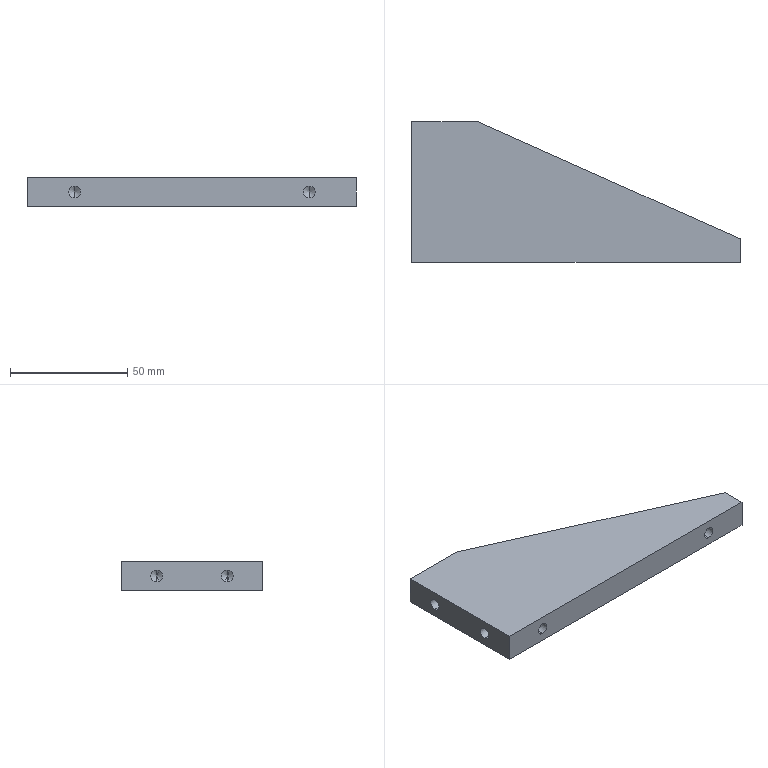Part | SolidWorks | features HoleWzd 3, Extrusion 1 | 1 solid | 27 faces | box 140 x 60 x 12 mm | volume 65678 mm3 | cylinder 10 | cone 10 | plane 7 | commonest cylinder face diameters 5 x10
STEP:
#1=CARTESIAN_POINT('',(20.,-15.,3.5));
#2=VERTEX_POINT('',#1);
#3=CARTESIAN_POINT('',(20.,-15.,8.5));
#4=VERTEX_POINT('',#3);
#5=CARTESIAN_POINT('',(20.,-15.,6.));
#6=DIRECTION('',(0.,1.,0.));
#7=DIRECTION('',(0.,0.,1.));
#8=AXIS2_PLACEMENT_3D('',#5,#6,#7);
#9=CIRCLE('',#8,2.5);
#10=EDGE_CURVE('',#2,#4,#9,.T.);
#11=ORIENTED_EDGE('',*,*,#10,.F.);
#12=CARTESIAN_POINT('',(20.,0.,3.5));
#13=VERTEX_POINT('',#12);
#14=CARTESIAN_POINT('',(20.,0.,3.5));
#15=DIRECTION('',(0.,1.,0.));
#16=VECTOR('',#15,1000.);
#17=LINE('',#14,#16);
#18=EDGE_CURVE('',#2,#13,#17,.T.);
#19=ORIENTED_EDGE('',*,*,#18,.T.);
#20=CARTESIAN_POINT('',(20.,0.,8.5));
#21=VERTEX_POINT('',#20);
#22=CARTESIAN_POINT('',(20.,0.,6.));
#23=DIRECTION('',(0.,1.,0.));
#24=DIRECTION('',(0.,0.,1.));
#25=AXIS2_PLACEMENT_3D('',#22,#23,#24);
#26=CIRCLE('',#25,2.5);
#27=EDGE_CURVE('',#13,#21,#26,.T.);
#28=ORIENTED_EDGE('',*,*,#27,.T.);
#29=CARTESIAN_POINT('',(20.,0.,8.5));
#30=DIRECTION('',(0.,1.,0.));
#31=VECTOR('',#30,1000.);
#32=LINE('',#29,#31);
#33=EDGE_CURVE('',#4,#21,#32,.T.);
#34=ORIENTED_EDGE('',*,*,#33,.F.);
#35=EDGE_LOOP('',(#11,#19,#28,#34));
#36=FACE_OUTER_BOUND('',#35,.T.);
#37=CARTESIAN_POINT('',(20.,0.,6.));
#38=DIRECTION('',(0.,1.,0.));
#39=DIRECTION('',(0.,0.,1.));
#40=AXIS2_PLACEMENT_3D('',#37,#38,#39);
#41=CYLINDRICAL_SURFACE('',#40,2.5);
#42=ADVANCED_FACE('',(#36),#41,.F.);
#43=CARTESIAN_POINT('',(20.,-16.502,6.));
#44=VERTEX_POINT('',#43);
#45=CARTESIAN_POINT('',(20.,-15.,8.5));
#46=DIRECTION('',(0.,0.515,0.8572));
#47=VECTOR('',#46,1000.);
#48=LINE('',#45,#47);
#49=EDGE_CURVE('',#44,#4,#48,.T.);
#50=ORIENTED_EDGE('',*,*,#49,.F.);
#51=CARTESIAN_POINT('',(20.,-15.,3.5));
#52=DIRECTION('',(0.,0.515,-0.8572));
#53=VECTOR('',#52,1000.);
#54=LINE('',#51,#53);
#55=EDGE_CURVE('',#44,#2,#54,.T.);
#56=ORIENTED_EDGE('',*,*,#55,.T.);
#57=ORIENTED_EDGE('',*,*,#10,.T.);
#58=EDGE_LOOP('',(#50,#56,#57));
#59=FACE_OUTER_BOUND('',#58,.T.);
#60=CARTESIAN_POINT('',(20.,-15.,6.));
#61=DIRECTION('',(0.,1.,0.));
#62=DIRECTION('',(0.,0.,1.));
#63=AXIS2_PLACEMENT_3D('',#60,#61,#62);
#64=CONICAL_SURFACE('',#63,2.5,1.03);
#65=ADVANCED_FACE('',(#59),#64,.F.);
#66=CARTESIAN_POINT('',(120.,-45.,8.5));
#67=VERTEX_POINT('',#66);
#68=CARTESIAN_POINT('',(120.,-45.,3.5));
#69=VERTEX_POINT('',#68);
#70=CARTESIAN_POINT('',(120.,-45.,6.));
#71=DIRECTION('',(0.,-1.,0.));
#72=DIRECTION('',(0.,0.,-1.));
#73=AXIS2_PLACEMENT_3D('',#70,#71,#72);
#74=CIRCLE('',#73,2.5);
#75=EDGE_CURVE('',#67,#69,#74,.T.);
#76=ORIENTED_EDGE('',*,*,#75,.F.);
#77=CARTESIAN_POINT('',(120.,-60.,8.5));
#78=VERTEX_POINT('',#77);
#79=CARTESIAN_POINT('',(120.,-60.,8.5));
#80=DIRECTION('',(0.,-1.,0.));
#81=VECTOR('',#80,1000.);
#82=LINE('',#79,#81);
#83=EDGE_CURVE('',#67,#78,#82,.T.);
#84=ORIENTED_EDGE('',*,*,#83,.T.);
#85=CARTESIAN_POINT('',(120.,-60.,3.5));
#86=VERTEX_POINT('',#85);
#87=CARTESIAN_POINT('',(120.,-60.,6.));
#88=DIRECTION('',(0.,-1.,0.));
#89=DIRECTION('',(0.,0.,-1.));
#90=AXIS2_PLACEMENT_3D('',#87,#88,#89);
#91=CIRCLE('',#90,2.5);
#92=EDGE_CURVE('',#78,#86,#91,.T.);
#93=ORIENTED_EDGE('',*,*,#92,.T.);
#94=CARTESIAN_POINT('',(120.,-60.,3.5));
#95=DIRECTION('',(0.,-1.,0.));
#96=VECTOR('',#95,1000.);
#97=LINE('',#94,#96);
#98=EDGE_CURVE('',#69,#86,#97,.T.);
#99=ORIENTED_EDGE('',*,*,#98,.F.);
#100=EDGE_LOOP('',(#76,#84,#93,#99));
#101=FACE_OUTER_BOUND('',#100,.T.);
#102=CARTESIAN_POINT('',(120.,-60.,6.));
#103=DIRECTION('',(0.,-1.,0.));
#104=DIRECTION('',(0.,0.,-1.));
#105=AXIS2_PLACEMENT_3D('',#102,#103,#104);
#106=CYLINDRICAL_SURFACE('',#105,2.5);
#107=ADVANCED_FACE('',(#101),#106,.F.);
#108=CARTESIAN_POINT('',(120.,-43.498,6.));
#109=VERTEX_POINT('',#108);
#110=CARTESIAN_POINT('',(120.,-45.,3.5));
#111=DIRECTION('',(0.,-0.515,-0.8572));
#112=VECTOR('',#111,1000.);
#113=LINE('',#110,#112);
#114=EDGE_CURVE('',#109,#69,#113,.T.);
#115=ORIENTED_EDGE('',*,*,#114,.F.);
#116=CARTESIAN_POINT('',(120.,-45.,8.5));
#117=DIRECTION('',(0.,-0.515,0.8572));
#118=VECTOR('',#117,1000.);
#119=LINE('',#116,#118);
#120=EDGE_CURVE('',#109,#67,#119,.T.);
#121=ORIENTED_EDGE('',*,*,#120,.T.);
#122=ORIENTED_EDGE('',*,*,#75,.T.);
#123=EDGE_LOOP('',(#115,#121,#122));
#124=FACE_OUTER_BOUND('',#123,.T.);
#125=CARTESIAN_POINT('',(120.,-45.,6.));
#126=DIRECTION('',(0.,-1.,0.));
#127=DIRECTION('',(0.,0.,-1.));
#128=AXIS2_PLACEMENT_3D('',#125,#126,#127);
#129=CONICAL_SURFACE('',#128,2.5,1.03);
#130=ADVANCED_FACE('',(#124),#129,.F.);
#131=CARTESIAN_POINT('',(20.,-45.,8.5));
#132=VERTEX_POINT('',#131);
#133=CARTESIAN_POINT('',(20.,-45.,3.5));
#134=VERTEX_POINT('',#133);
#135=CARTESIAN_POINT('',(20.,-45.,6.));
#136=DIRECTION('',(0.,-1.,0.));
#137=DIRECTION('',(0.,0.,-1.));
#138=AXIS2_PLACEMENT_3D('',#135,#136,#137);
#139=CIRCLE('',#138,2.5);
#140=EDGE_CURVE('',#132,#134,#139,.T.);
#141=ORIENTED_EDGE('',*,*,#140,.F.);
#142=CARTESIAN_POINT('',(20.,-60.,8.5));
#143=VERTEX_POINT('',#142);
#144=CARTESIAN_POINT('',(20.,-60.,8.5));
#145=DIRECTION('',(0.,-1.,0.));
#146=VECTOR('',#145,1000.);
#147=LINE('',#144,#146);
#148=EDGE_CURVE('',#132,#143,#147,.T.);
#149=ORIENTED_EDGE('',*,*,#148,.T.);
#150=CARTESIAN_POINT('',(20.,-60.,3.5));
#151=VERTEX_POINT('',#150);
#152=CARTESIAN_POINT('',(20.,-60.,6.));
#153=DIRECTION('',(0.,-1.,0.));
#154=DIRECTION('',(0.,0.,-1.));
#155=AXIS2_PLACEMENT_3D('',#152,#153,#154);
#156=CIRCLE('',#155,2.5);
#157=EDGE_CURVE('',#143,#151,#156,.T.);
#158=ORIENTED_EDGE('',*,*,#157,.T.);
#159=CARTESIAN_POINT('',(20.,-60.,3.5));
#160=DIRECTION('',(0.,-1.,0.));
#161=VECTOR('',#160,1000.);
#162=LINE('',#159,#161);
#163=EDGE_CURVE('',#134,#151,#162,.T.);
#164=ORIENTED_EDGE('',*,*,#163,.F.);
#165=EDGE_LOOP('',(#141,#149,#158,#164));
#166=FACE_OUTER_BOUND('',#165,.T.);
#167=CARTESIAN_POINT('',(20.,-60.,6.));
#168=DIRECTION('',(0.,-1.,0.));
#169=DIRECTION('',(0.,0.,-1.));
#170=AXIS2_PLACEMENT_3D('',#167,#168,#169);
#171=CYLINDRICAL_SURFACE('',#170,2.5);
#172=ADVANCED_FACE('',(#166),#171,.F.);
#173=CARTESIAN_POINT('',(20.,-43.498,6.));
#174=VERTEX_POINT('',#173);
#175=CARTESIAN_POINT('',(20.,-45.,3.5));
#176=DIRECTION('',(0.,-0.515,-0.8572));
#177=VECTOR('',#176,1000.);
#178=LINE('',#175,#177);
#179=EDGE_CURVE('',#174,#134,#178,.T.);
#180=ORIENTED_EDGE('',*,*,#179,.F.);
#181=CARTESIAN_POINT('',(20.,-45.,8.5));
#182=DIRECTION('',(0.,-0.515,0.8572));
#183=VECTOR('',#182,1000.);
#184=LINE('',#181,#183);
#185=EDGE_CURVE('',#174,#132,#184,.T.);
#186=ORIENTED_EDGE('',*,*,#185,.T.);
#187=ORIENTED_EDGE('',*,*,#140,.T.);
#188=EDGE_LOOP('',(#180,#186,#187));
#189=FACE_OUTER_BOUND('',#188,.T.);
#190=CARTESIAN_POINT('',(20.,-45.,6.));
#191=DIRECTION('',(0.,-1.,0.));
#192=DIRECTION('',(0.,0.,-1.));
#193=AXIS2_PLACEMENT_3D('',#190,#191,#192);
#194=CONICAL_SURFACE('',#193,2.5,1.03);
#195=ADVANCED_FACE('',(#189),#194,.F.);
#196=CARTESIAN_POINT('',(15.,-15.,3.5));
#197=VERTEX_POINT('',#196);
#198=CARTESIAN_POINT('',(15.,-15.,8.5));
#199=VERTEX_POINT('',#198);
#200=CARTESIAN_POINT('',(15.,-15.,6.));
#201=DIRECTION('',(-1.,0.,0.));
#202=DIRECTION('',(0.,0.,1.));
#203=AXIS2_PLACEMENT_3D('',#200,#201,#202);
#204=CIRCLE('',#203,2.5);
#205=EDGE_CURVE('',#197,#199,#204,.T.);
#206=ORIENTED_EDGE('',*,*,#205,.F.);
#207=CARTESIAN_POINT('',(0.,-15.,3.5));
#208=VERTEX_POINT('',#207);
#209=CARTESIAN_POINT('',(0.,-15.,3.5));
#210=DIRECTION('',(-1.,0.,0.));
#211=VECTOR('',#210,1000.);
#212=LINE('',#209,#211);
#213=EDGE_CURVE('',#197,#208,#212,.T.);
#214=ORIENTED_EDGE('',*,*,#213,.T.);
#215=CARTESIAN_POINT('',(0.,-15.,8.5));
#216=VERTEX_POINT('',#215);
#217=CARTESIAN_POINT('',(0.,-15.,6.));
#218=DIRECTION('',(-1.,0.,0.));
#219=DIRECTION('',(0.,0.,1.));
#220=AXIS2_PLACEMENT_3D('',#217,#218,#219);
#221=CIRCLE('',#220,2.5);
#222=EDGE_CURVE('',#208,#216,#221,.T.);
#223=ORIENTED_EDGE('',*,*,#222,.T.);
#224=CARTESIAN_POINT('',(0.,-15.,8.5));
#225=DIRECTION('',(-1.,0.,0.));
#226=VECTOR('',#225,1000.);
#227=LINE('',#224,#226);
#228=EDGE_CURVE('',#199,#216,#227,.T.);
#229=ORIENTED_EDGE('',*,*,#228,.F.);
#230=EDGE_LOOP('',(#206,#214,#223,#229));
#231=FACE_OUTER_BOUND('',#230,.T.);
#232=CARTESIAN_POINT('',(0.,-15.,6.));
#233=DIRECTION('',(-1.,0.,0.));
#234=DIRECTION('',(0.,0.,1.));
#235=AXIS2_PLACEMENT_3D('',#232,#233,#234);
#236=CYLINDRICAL_SURFACE('',#235,2.5);
#237=ADVANCED_FACE('',(#231),#236,.F.);
#238=CARTESIAN_POINT('',(16.502,-15.,6.));
#239=VERTEX_POINT('',#238);
#240=CARTESIAN_POINT('',(15.,-15.,8.5));
#241=DIRECTION('',(-0.515,0.,0.8572));
#242=VECTOR('',#241,1000.);
#243=LINE('',#240,#242);
#244=EDGE_CURVE('',#239,#199,#243,.T.);
#245=ORIENTED_EDGE('',*,*,#244,.F.);
#246=CARTESIAN_POINT('',(15.,-15.,3.5));
#247=DIRECTION('',(-0.515,0.,-0.8572));
#248=VECTOR('',#247,1000.);
#249=LINE('',#246,#248);
#250=EDGE_CURVE('',#239,#197,#249,.T.);
#251=ORIENTED_EDGE('',*,*,#250,.T.);
#252=ORIENTED_EDGE('',*,*,#205,.T.);
#253=EDGE_LOOP('',(#245,#251,#252));
#254=FACE_OUTER_BOUND('',#253,.T.);
#255=CARTESIAN_POINT('',(15.,-15.,6.));
#256=DIRECTION('',(-1.,0.,0.));
#257=DIRECTION('',(0.,0.,1.));
#258=AXIS2_PLACEMENT_3D('',#255,#256,#257);
#259=CONICAL_SURFACE('',#258,2.5,1.03);
#260=ADVANCED_FACE('',(#254),#259,.F.);
#261=CARTESIAN_POINT('',(15.,-45.,3.5));
#262=VERTEX_POINT('',#261);
#263=CARTESIAN_POINT('',(15.,-45.,8.5));
#264=VERTEX_POINT('',#263);
#265=CARTESIAN_POINT('',(15.,-45.,6.));
#266=DIRECTION('',(-1.,0.,0.));
#267=DIRECTION('',(0.,0.,1.));
#268=AXIS2_PLACEMENT_3D('',#265,#266,#267);
#269=CIRCLE('',#268,2.5);
#270=EDGE_CURVE('',#262,#264,#269,.T.);
#271=ORIENTED_EDGE('',*,*,#270,.F.);
#272=CARTESIAN_POINT('',(0.,-45.,3.5));
#273=VERTEX_POINT('',#272);
#274=CARTESIAN_POINT('',(0.,-45.,3.5));
#275=DIRECTION('',(-1.,0.,0.));
#276=VECTOR('',#275,1000.);
#277=LINE('',#274,#276);
#278=EDGE_CURVE('',#262,#273,#277,.T.);
#279=ORIENTED_EDGE('',*,*,#278,.T.);
#280=CARTESIAN_POINT('',(0.,-45.,8.5));
#281=VERTEX_POINT('',#280);
#282=CARTESIAN_POINT('',(0.,-45.,6.));
#283=DIRECTION('',(-1.,0.,0.));
#284=DIRECTION('',(0.,0.,1.));
#285=AXIS2_PLACEMENT_3D('',#282,#283,#284);
#286=CIRCLE('',#285,2.5);
#287=EDGE_CURVE('',#273,#281,#286,.T.);
#288=ORIENTED_EDGE('',*,*,#287,.T.);
#289=CARTESIAN_POINT('',(0.,-45.,8.5));
#290=DIRECTION('',(-1.,0.,0.));
#291=VECTOR('',#290,1000.);
#292=LINE('',#289,#291);
#293=EDGE_CURVE('',#264,#281,#292,.T.);
#294=ORIENTED_EDGE('',*,*,#293,.F.);
#295=EDGE_LOOP('',(#271,#279,#288,#294));
#296=FACE_OUTER_BOUND('',#295,.T.);
#297=CARTESIAN_POINT('',(0.,-45.,6.));
#298=DIRECTION('',(-1.,0.,0.));
#299=DIRECTION('',(0.,0.,1.));
#300=AXIS2_PLACEMENT_3D('',#297,#298,#299);
#301=CYLINDRICAL_SURFACE('',#300,2.5);
#302=ADVANCED_FACE('',(#296),#301,.F.);
#303=CARTESIAN_POINT('',(16.502,-45.,6.));
#304=VERTEX_POINT('',#303);
#305=CARTESIAN_POINT('',(15.,-45.,8.5));
#306=DIRECTION('',(-0.515,0.,0.8572));
#307=VECTOR('',#306,1000.);
#308=LINE('',#305,#307);
#309=EDGE_CURVE('',#304,#264,#308,.T.);
#310=ORIENTED_EDGE('',*,*,#309,.F.);
#311=CARTESIAN_POINT('',(15.,-45.,3.5));
#312=DIRECTION('',(-0.515,0.,-0.8572));
#313=VECTOR('',#312,1000.);
#314=LINE('',#311,#313);
#315=EDGE_CURVE('',#304,#262,#314,.T.);
#316=ORIENTED_EDGE('',*,*,#315,.T.);
#317=ORIENTED_EDGE('',*,*,#270,.T.);
#318=EDGE_LOOP('',(#310,#316,#317));
#319=FACE_OUTER_BOUND('',#318,.T.);
#320=CARTESIAN_POINT('',(15.,-45.,6.));
#321=DIRECTION('',(-1.,0.,0.));
#322=DIRECTION('',(0.,0.,1.));
#323=AXIS2_PLACEMENT_3D('',#320,#321,#322);
#324=CONICAL_SURFACE('',#323,2.5,1.03);
#325=ADVANCED_FACE('',(#319),#324,.F.);
#326=CARTESIAN_POINT('',(20.,0.,6.));
#327=DIRECTION('',(0.,1.,0.));
#328=DIRECTION('',(0.,0.,1.));
#329=AXIS2_PLACEMENT_3D('',#326,#327,#328);
#330=CIRCLE('',#329,2.5);
#331=EDGE_CURVE('',#21,#13,#330,.T.);
#332=ORIENTED_EDGE('',*,*,#331,.F.);
#333=ORIENTED_EDGE('',*,*,#27,.F.);
#334=EDGE_LOOP('',(#332,#333));
#335=FACE_BOUND('',#334,.T.);
#336=CARTESIAN_POINT('',(28.,0.,0.));
#337=VERTEX_POINT('',#336);
#338=CARTESIAN_POINT('',(0.,0.,0.));
#339=VERTEX_POINT('',#338);
#340=CARTESIAN_POINT('',(28.,0.,0.));
#341=DIRECTION('',(-1.,0.,0.));
#342=VECTOR('',#341,1000.);
#343=LINE('',#340,#342);
#344=EDGE_CURVE('',#337,#339,#343,.T.);
#345=ORIENTED_EDGE('',*,*,#344,.T.);
#346=CARTESIAN_POINT('',(0.,0.,12.));
#347=VERTEX_POINT('',#346);
#348=CARTESIAN_POINT('',(0.,0.,12.));
#349=DIRECTION('',(0.,0.,-1.));
#350=VECTOR('',#349,1000.);
#351=LINE('',#348,#350);
#352=EDGE_CURVE('',#347,#339,#351,.T.);
#353=ORIENTED_EDGE('',*,*,#352,.F.);
#354=CARTESIAN_POINT('',(28.,0.,12.));
#355=VERTEX_POINT('',#354);
#356=CARTESIAN_POINT('',(28.,0.,12.));
#357=DIRECTION('',(-1.,0.,0.));
#358=VECTOR('',#357,1000.);
#359=LINE('',#356,#358);
#360=EDGE_CURVE('',#355,#347,#359,.T.);
#361=ORIENTED_EDGE('',*,*,#360,.F.);
#362=CARTESIAN_POINT('',(28.,0.,12.));
#363=DIRECTION('',(0.,0.,-1.));
#364=VECTOR('',#363,1000.);
#365=LINE('',#362,#364);
#366=EDGE_CURVE('',#355,#337,#365,.T.);
#367=ORIENTED_EDGE('',*,*,#366,.T.);
#368=EDGE_LOOP('',(#345,#353,#361,#367));
#369=FACE_OUTER_BOUND('',#368,.T.);
#370=CARTESIAN_POINT('',(28.,0.,12.));
#371=DIRECTION('',(0.,-1.,0.));
#372=DIRECTION('',(1.,0.,0.));
#373=AXIS2_PLACEMENT_3D('',#370,#371,#372);
#374=PLANE('',#373);
#375=ADVANCED_FACE('',(#335,#369),#374,.F.);
#376=CARTESIAN_POINT('',(0.,-15.,6.));
#377=DIRECTION('',(-1.,0.,0.));
#378=DIRECTION('',(0.,0.,1.));
#379=AXIS2_PLACEMENT_3D('',#376,#377,#378);
#380=CIRCLE('',#379,2.5);
#381=EDGE_CURVE('',#216,#208,#380,.T.);
#382=ORIENTED_EDGE('',*,*,#381,.F.);
#383=ORIENTED_EDGE('',*,*,#222,.F.);
#384=EDGE_LOOP('',(#382,#383));
#385=FACE_BOUND('',#384,.T.);
#386=CARTESIAN_POINT('',(0.,-45.,6.));
#387=DIRECTION('',(-1.,0.,0.));
#388=DIRECTION('',(0.,0.,1.));
#389=AXIS2_PLACEMENT_3D('',#386,#387,#388);
#390=CIRCLE('',#389,2.5);
#391=EDGE_CURVE('',#281,#273,#390,.T.);
#392=ORIENTED_EDGE('',*,*,#391,.F.);
#393=ORIENTED_EDGE('',*,*,#287,.F.);
#394=EDGE_LOOP('',(#392,#393));
#395=FACE_BOUND('',#394,.T.);
#396=CARTESIAN_POINT('',(0.,-60.,0.));
#397=VERTEX_POINT('',#396);
#398=CARTESIAN_POINT('',(0.,0.,0.));
#399=DIRECTION('',(0.,-1.,0.));
#400=VECTOR('',#399,1000.);
#401=LINE('',#398,#400);
#402=EDGE_CURVE('',#339,#397,#401,.T.);
#403=ORIENTED_EDGE('',*,*,#402,.T.);
#404=CARTESIAN_POINT('',(0.,-60.,12.));
#405=VERTEX_POINT('',#404);
#406=CARTESIAN_POINT('',(0.,-60.,12.));
#407=DIRECTION('',(0.,0.,-1.));
#408=VECTOR('',#407,1000.);
#409=LINE('',#406,#408);
#410=EDGE_CURVE('',#405,#397,#409,.T.);
#411=ORIENTED_EDGE('',*,*,#410,.F.);
#412=CARTESIAN_POINT('',(0.,0.,12.));
#413=DIRECTION('',(0.,-1.,0.));
#414=VECTOR('',#413,1000.);
#415=LINE('',#412,#414);
#416=EDGE_CURVE('',#347,#405,#415,.T.);
#417=ORIENTED_EDGE('',*,*,#416,.F.);
#418=ORIENTED_EDGE('',*,*,#352,.T.);
#419=EDGE_LOOP('',(#403,#411,#417,#418));
#420=FACE_OUTER_BOUND('',#419,.T.);
#421=CARTESIAN_POINT('',(0.,0.,12.));
#422=DIRECTION('',(1.,0.,0.));
#423=DIRECTION('',(0.,1.,0.));
#424=AXIS2_PLACEMENT_3D('',#421,#422,#423);
#425=PLANE('',#424);
#426=ADVANCED_FACE('',(#385,#395,#420),#425,.F.);
#427=CARTESIAN_POINT('',(120.,-60.,6.));
#428=DIRECTION('',(0.,-1.,0.));
#429=DIRECTION('',(0.,0.,-1.));
#430=AXIS2_PLACEMENT_3D('',#427,#428,#429);
#431=CIRCLE('',#430,2.5);
#432=EDGE_CURVE('',#86,#78,#431,.T.);
#433=ORIENTED_EDGE('',*,*,#432,.F.);
#434=ORIENTED_EDGE('',*,*,#92,.F.);
#435=EDGE_LOOP('',(#433,#434));
#436=FACE_BOUND('',#435,.T.);
#437=CARTESIAN_POINT('',(20.,-60.,6.));
#438=DIRECTION('',(0.,-1.,0.));
#439=DIRECTION('',(0.,0.,-1.));
#440=AXIS2_PLACEMENT_3D('',#437,#438,#439);
#441=CIRCLE('',#440,2.5);
#442=EDGE_CURVE('',#151,#143,#441,.T.);
#443=ORIENTED_EDGE('',*,*,#442,.F.);
#444=ORIENTED_EDGE('',*,*,#157,.F.);
#445=EDGE_LOOP('',(#443,#444));
#446=FACE_BOUND('',#445,.T.);
#447=CARTESIAN_POINT('',(140.,-60.,0.));
#448=VERTEX_POINT('',#447);
#449=CARTESIAN_POINT('',(0.,-60.,0.));
#450=DIRECTION('',(1.,0.,0.));
#451=VECTOR('',#450,1000.);
#452=LINE('',#449,#451);
#453=EDGE_CURVE('',#397,#448,#452,.T.);
#454=ORIENTED_EDGE('',*,*,#453,.T.);
#455=CARTESIAN_POINT('',(140.,-60.,12.));
#456=VERTEX_POINT('',#455);
#457=CARTESIAN_POINT('',(140.,-60.,12.));
#458=DIRECTION('',(0.,0.,-1.));
#459=VECTOR('',#458,1000.);
#460=LINE('',#457,#459);
#461=EDGE_CURVE('',#456,#448,#460,.T.);
#462=ORIENTED_EDGE('',*,*,#461,.F.);
#463=CARTESIAN_POINT('',(0.,-60.,12.));
#464=DIRECTION('',(1.,0.,0.));
#465=VECTOR('',#464,1000.);
#466=LINE('',#463,#465);
#467=EDGE_CURVE('',#405,#456,#466,.T.);
#468=ORIENTED_EDGE('',*,*,#467,.F.);
#469=ORIENTED_EDGE('',*,*,#410,.T.);
#470=EDGE_LOOP('',(#454,#462,#468,#469));
#471=FACE_OUTER_BOUND('',#470,.T.);
#472=CARTESIAN_POINT('',(0.,-60.,12.));
#473=DIRECTION('',(0.,1.,0.));
#474=DIRECTION('',(0.,0.,1.));
#475=AXIS2_PLACEMENT_3D('',#472,#473,#474);
#476=PLANE('',#475);
#477=ADVANCED_FACE('',(#436,#446,#471),#476,.F.);
#478=CARTESIAN_POINT('',(140.,-50.,0.));
#479=VERTEX_POINT('',#478);
#480=CARTESIAN_POINT('',(140.,-60.,0.));
#481=DIRECTION('',(0.,1.,0.));
#482=VECTOR('',#481,1000.);
#483=LINE('',#480,#482);
#484=EDGE_CURVE('',#448,#479,#483,.T.);
#485=ORIENTED_EDGE('',*,*,#484,.T.);
#486=CARTESIAN_POINT('',(140.,-50.,12.));
#487=VERTEX_POINT('',#486);
#488=CARTESIAN_POINT('',(140.,-50.,12.));
#489=DIRECTION('',(0.,0.,-1.));
#490=VECTOR('',#489,1000.);
#491=LINE('',#488,#490);
#492=EDGE_CURVE('',#487,#479,#491,.T.);
#493=ORIENTED_EDGE('',*,*,#492,.F.);
#494=CARTESIAN_POINT('',(140.,-60.,12.));
#495=DIRECTION('',(0.,1.,0.));
#496=VECTOR('',#495,1000.);
#497=LINE('',#494,#496);
#498=EDGE_CURVE('',#456,#487,#497,.T.);
#499=ORIENTED_EDGE('',*,*,#498,.F.);
#500=ORIENTED_EDGE('',*,*,#461,.T.);
#501=EDGE_LOOP('',(#485,#493,#499,#500));
#502=FACE_OUTER_BOUND('',#501,.T.);
#503=CARTESIAN_POINT('',(140.,-60.,12.));
#504=DIRECTION('',(-1.,0.,0.));
#505=DIRECTION('',(0.,0.,1.));
#506=AXIS2_PLACEMENT_3D('',#503,#504,#505);
#507=PLANE('',#506);
#508=ADVANCED_FACE('',(#502),#507,.F.);
#509=CARTESIAN_POINT('',(140.,-50.,0.));
#510=DIRECTION('',(-0.9131,0.4077,0.));
#511=VECTOR('',#510,1000.);
#512=LINE('',#509,#511);
#513=EDGE_CURVE('',#479,#337,#512,.T.);
#514=ORIENTED_EDGE('',*,*,#513,.T.);
#515=ORIENTED_EDGE('',*,*,#366,.F.);
#516=CARTESIAN_POINT('',(140.,-50.,12.));
#517=DIRECTION('',(-0.9131,0.4077,0.));
#518=VECTOR('',#517,1000.);
#519=LINE('',#516,#518);
#520=EDGE_CURVE('',#487,#355,#519,.T.);
#521=ORIENTED_EDGE('',*,*,#520,.F.);
#522=ORIENTED_EDGE('',*,*,#492,.T.);
#523=EDGE_LOOP('',(#514,#515,#521,#522));
#524=FACE_OUTER_BOUND('',#523,.T.);
#525=CARTESIAN_POINT('',(140.,-50.,12.));
#526=DIRECTION('',(-0.4077,-0.9131,0.));
#527=DIRECTION('',(0.9131,-0.4077,0.));
#528=AXIS2_PLACEMENT_3D('',#525,#526,#527);
#529=PLANE('',#528);
#530=ADVANCED_FACE('',(#524),#529,.F.);
#531=ORIENTED_EDGE('',*,*,#360,.T.);
#532=ORIENTED_EDGE('',*,*,#416,.T.);
#533=ORIENTED_EDGE('',*,*,#467,.T.);
#534=ORIENTED_EDGE('',*,*,#498,.T.);
#535=ORIENTED_EDGE('',*,*,#520,.T.);
#536=EDGE_LOOP('',(#531,#532,#533,#534,#535));
#537=FACE_OUTER_BOUND('',#536,.T.);
#538=CARTESIAN_POINT('',(0.,0.,12.));
#539=DIRECTION('',(0.,0.,1.));
#540=DIRECTION('',(1.,0.,0.));
#541=AXIS2_PLACEMENT_3D('',#538,#539,#540);
#542=PLANE('',#541);
#543=ADVANCED_FACE('',(#537),#542,.T.);
#544=ORIENTED_EDGE('',*,*,#344,.F.);
#545=ORIENTED_EDGE('',*,*,#513,.F.);
#546=ORIENTED_EDGE('',*,*,#484,.F.);
#547=ORIENTED_EDGE('',*,*,#453,.F.);
#548=ORIENTED_EDGE('',*,*,#402,.F.);
#549=EDGE_LOOP('',(#544,#545,#546,#547,#548));
#550=FACE_OUTER_BOUND('',#549,.T.);
#551=CARTESIAN_POINT('',(0.,0.,0.));
#552=DIRECTION('',(0.,0.,1.));
#553=DIRECTION('',(1.,0.,0.));
#554=AXIS2_PLACEMENT_3D('',#551,#552,#553);
#555=PLANE('',#554);
#556=ADVANCED_FACE('',(#550),#555,.F.);
#557=ORIENTED_EDGE('',*,*,#315,.F.);
#558=ORIENTED_EDGE('',*,*,#309,.T.);
#559=CARTESIAN_POINT('',(15.,-45.,6.));
#560=DIRECTION('',(-1.,0.,0.));
#561=DIRECTION('',(0.,0.,1.));
#562=AXIS2_PLACEMENT_3D('',#559,#560,#561);
#563=CIRCLE('',#562,2.5);
#564=EDGE_CURVE('',#264,#262,#563,.T.);
#565=ORIENTED_EDGE('',*,*,#564,.T.);
#566=EDGE_LOOP('',(#557,#558,#565));
#567=FACE_OUTER_BOUND('',#566,.T.);
#568=CARTESIAN_POINT('',(15.,-45.,6.));
#569=DIRECTION('',(-1.,0.,0.));
#570=DIRECTION('',(0.,0.,1.));
#571=AXIS2_PLACEMENT_3D('',#568,#569,#570);
#572=CONICAL_SURFACE('',#571,2.5,1.03);
#573=ADVANCED_FACE('',(#567),#572,.F.);
#574=ORIENTED_EDGE('',*,*,#278,.F.);
#575=ORIENTED_EDGE('',*,*,#564,.F.);
#576=ORIENTED_EDGE('',*,*,#293,.T.);
#577=ORIENTED_EDGE('',*,*,#391,.T.);
#578=EDGE_LOOP('',(#574,#575,#576,#577));
#579=FACE_OUTER_BOUND('',#578,.T.);
#580=CARTESIAN_POINT('',(0.,-45.,6.));
#581=DIRECTION('',(-1.,0.,0.));
#582=DIRECTION('',(0.,0.,1.));
#583=AXIS2_PLACEMENT_3D('',#580,#581,#582);
#584=CYLINDRICAL_SURFACE('',#583,2.5);
#585=ADVANCED_FACE('',(#579),#584,.F.);
#586=ORIENTED_EDGE('',*,*,#250,.F.);
#587=ORIENTED_EDGE('',*,*,#244,.T.);
#588=CARTESIAN_POINT('',(15.,-15.,6.));
#589=DIRECTION('',(-1.,0.,0.));
#590=DIRECTION('',(0.,0.,1.));
#591=AXIS2_PLACEMENT_3D('',#588,#589,#590);
#592=CIRCLE('',#591,2.5);
#593=EDGE_CURVE('',#199,#197,#592,.T.);
#594=ORIENTED_EDGE('',*,*,#593,.T.);
#595=EDGE_LOOP('',(#586,#587,#594));
#596=FACE_OUTER_BOUND('',#595,.T.);
#597=CARTESIAN_POINT('',(15.,-15.,6.));
#598=DIRECTION('',(-1.,0.,0.));
#599=DIRECTION('',(0.,0.,1.));
#600=AXIS2_PLACEMENT_3D('',#597,#598,#599);
#601=CONICAL_SURFACE('',#600,2.5,1.03);
#602=ADVANCED_FACE('',(#596),#601,.F.);
#603=ORIENTED_EDGE('',*,*,#213,.F.);
#604=ORIENTED_EDGE('',*,*,#593,.F.);
#605=ORIENTED_EDGE('',*,*,#228,.T.);
#606=ORIENTED_EDGE('',*,*,#381,.T.);
#607=EDGE_LOOP('',(#603,#604,#605,#606));
#608=FACE_OUTER_BOUND('',#607,.T.);
#609=CARTESIAN_POINT('',(0.,-15.,6.));
#610=DIRECTION('',(-1.,0.,0.));
#611=DIRECTION('',(0.,0.,1.));
#612=AXIS2_PLACEMENT_3D('',#609,#610,#611);
#613=CYLINDRICAL_SURFACE('',#612,2.5);
#614=ADVANCED_FACE('',(#608),#613,.F.);
#615=ORIENTED_EDGE('',*,*,#185,.F.);
#616=ORIENTED_EDGE('',*,*,#179,.T.);
#617=CARTESIAN_POINT('',(20.,-45.,6.));
#618=DIRECTION('',(0.,-1.,0.));
#619=DIRECTION('',(0.,0.,-1.));
#620=AXIS2_PLACEMENT_3D('',#617,#618,#619);
#621=CIRCLE('',#620,2.5);
#622=EDGE_CURVE('',#134,#132,#621,.T.);
#623=ORIENTED_EDGE('',*,*,#622,.T.);
#624=EDGE_LOOP('',(#615,#616,#623));
#625=FACE_OUTER_BOUND('',#624,.T.);
#626=CARTESIAN_POINT('',(20.,-45.,6.));
#627=DIRECTION('',(0.,-1.,0.));
#628=DIRECTION('',(0.,0.,-1.));
#629=AXIS2_PLACEMENT_3D('',#626,#627,#628);
#630=CONICAL_SURFACE('',#629,2.5,1.03);
#631=ADVANCED_FACE('',(#625),#630,.F.);
#632=ORIENTED_EDGE('',*,*,#148,.F.);
#633=ORIENTED_EDGE('',*,*,#622,.F.);
#634=ORIENTED_EDGE('',*,*,#163,.T.);
#635=ORIENTED_EDGE('',*,*,#442,.T.);
#636=EDGE_LOOP('',(#632,#633,#634,#635));
#637=FACE_OUTER_BOUND('',#636,.T.);
#638=CARTESIAN_POINT('',(20.,-60.,6.));
#639=DIRECTION('',(0.,-1.,0.));
#640=DIRECTION('',(0.,0.,-1.));
#641=AXIS2_PLACEMENT_3D('',#638,#639,#640);
#642=CYLINDRICAL_SURFACE('',#641,2.5);
#643=ADVANCED_FACE('',(#637),#642,.F.);
#644=ORIENTED_EDGE('',*,*,#120,.F.);
#645=ORIENTED_EDGE('',*,*,#114,.T.);
#646=CARTESIAN_POINT('',(120.,-45.,6.));
#647=DIRECTION('',(0.,-1.,0.));
#648=DIRECTION('',(0.,0.,-1.));
#649=AXIS2_PLACEMENT_3D('',#646,#647,#648);
#650=CIRCLE('',#649,2.5);
#651=EDGE_CURVE('',#69,#67,#650,.T.);
#652=ORIENTED_EDGE('',*,*,#651,.T.);
#653=EDGE_LOOP('',(#644,#645,#652));
#654=FACE_OUTER_BOUND('',#653,.T.);
#655=CARTESIAN_POINT('',(120.,-45.,6.));
#656=DIRECTION('',(0.,-1.,0.));
#657=DIRECTION('',(0.,0.,-1.));
#658=AXIS2_PLACEMENT_3D('',#655,#656,#657);
#659=CONICAL_SURFACE('',#658,2.5,1.03);
#660=ADVANCED_FACE('',(#654),#659,.F.);
#661=ORIENTED_EDGE('',*,*,#83,.F.);
#662=ORIENTED_EDGE('',*,*,#651,.F.);
#663=ORIENTED_EDGE('',*,*,#98,.T.);
#664=ORIENTED_EDGE('',*,*,#432,.T.);
#665=EDGE_LOOP('',(#661,#662,#663,#664));
#666=FACE_OUTER_BOUND('',#665,.T.);
#667=CARTESIAN_POINT('',(120.,-60.,6.));
#668=DIRECTION('',(0.,-1.,0.));
#669=DIRECTION('',(0.,0.,-1.));
#670=AXIS2_PLACEMENT_3D('',#667,#668,#669);
#671=CYLINDRICAL_SURFACE('',#670,2.5);
#672=ADVANCED_FACE('',(#666),#671,.F.);
#673=ORIENTED_EDGE('',*,*,#55,.F.);
#674=ORIENTED_EDGE('',*,*,#49,.T.);
#675=CARTESIAN_POINT('',(20.,-15.,6.));
#676=DIRECTION('',(0.,1.,0.));
#677=DIRECTION('',(0.,0.,1.));
#678=AXIS2_PLACEMENT_3D('',#675,#676,#677);
#679=CIRCLE('',#678,2.5);
#680=EDGE_CURVE('',#4,#2,#679,.T.);
#681=ORIENTED_EDGE('',*,*,#680,.T.);
#682=EDGE_LOOP('',(#673,#674,#681));
#683=FACE_OUTER_BOUND('',#682,.T.);
#684=CARTESIAN_POINT('',(20.,-15.,6.));
#685=DIRECTION('',(0.,1.,0.));
#686=DIRECTION('',(0.,0.,1.));
#687=AXIS2_PLACEMENT_3D('',#684,#685,#686);
#688=CONICAL_SURFACE('',#687,2.5,1.03);
#689=ADVANCED_FACE('',(#683),#688,.F.);
#690=ORIENTED_EDGE('',*,*,#18,.F.);
#691=ORIENTED_EDGE('',*,*,#680,.F.);
#692=ORIENTED_EDGE('',*,*,#33,.T.);
#693=ORIENTED_EDGE('',*,*,#331,.T.);
#694=EDGE_LOOP('',(#690,#691,#692,#693));
#695=FACE_OUTER_BOUND('',#694,.T.);
#696=CARTESIAN_POINT('',(20.,0.,6.));
#697=DIRECTION('',(0.,1.,0.));
#698=DIRECTION('',(0.,0.,1.));
#699=AXIS2_PLACEMENT_3D('',#696,#697,#698);
#700=CYLINDRICAL_SURFACE('',#699,2.5);
#701=ADVANCED_FACE('',(#695),#700,.F.);
#702=CLOSED_SHELL('',(#42,#65,#107,#130,#172,#195,#237,#260,#302,#325,#375,#426,#477,#508,#530,#543,#556,#573,#585,#602,#614,#631,#643,#660,#672,#689,#701));
#703=MANIFOLD_SOLID_BREP('',#702);
#704=CARTESIAN_POINT('',(0.,0.,0.));
#705=DIRECTION('',(0.,0.,1.));
#706=DIRECTION('',(1.,0.,0.));
#707=AXIS2_PLACEMENT_3D('',#704,#705,#706);
#708=(LENGTH_UNIT()NAMED_UNIT(*)SI_UNIT(.MILLI.,.METRE.));
#709=UNCERTAINTY_MEASURE_WITH_UNIT(LENGTH_MEASURE(0.00001),#708,'','');
#710=(NAMED_UNIT(*)PLANE_ANGLE_UNIT()SI_UNIT($,.RADIAN.));
#711=(NAMED_UNIT(*)SI_UNIT($,.STERADIAN.)SOLID_ANGLE_UNIT());
#712=(GEOMETRIC_REPRESENTATION_CONTEXT(3)GLOBAL_UNCERTAINTY_ASSIGNED_CONTEXT((#709))GLOBAL_UNIT_ASSIGNED_CONTEXT((#708,#710,#711))REPRESENTATION_CONTEXT('',''));
#713=ADVANCED_BREP_SHAPE_REPRESENTATION('',(#703,#707),#712);